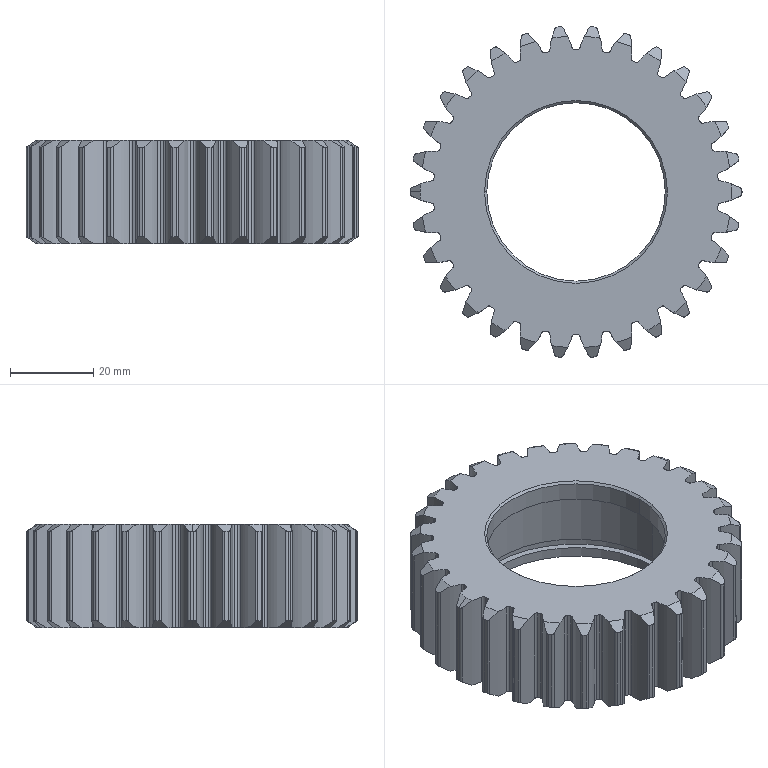Part | SolidWorks | features BaseBody 1 | 1 solid | 342 faces | box 80 x 79.651 x 25 mm | volume 58783 mm3 | cylinder 273 | cone 64 | plane 5 | commonest cylinder face diameters 1.25 x142 31.694 x62 80 x31 68.75 x30 52 x4 43 x2